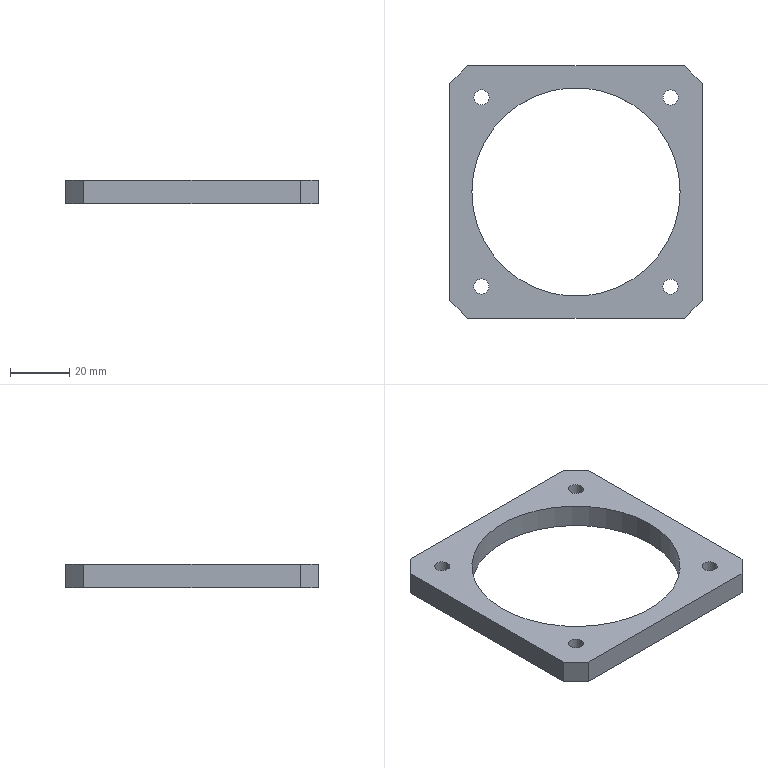Part | NX | 1 solid | 15 faces | box 85 x 85 x 8 mm | volume 25695 mm3 | plane 10 | cylinder 5 | commonest cylinder face diameters 5.1 x4 70.1 x1
STEP:
#1=CARTESIAN_POINT('',(-36.5,-42.5,0.));
#2=VERTEX_POINT('',#1);
#3=CARTESIAN_POINT('',(36.5,-42.5,0.));
#4=VERTEX_POINT('',#3);
#5=CARTESIAN_POINT('',(-36.5,-42.5,0.));
#6=DIRECTION('',(1.,0.,0.));
#7=VECTOR('',#6,1000.);
#8=LINE('',#5,#7);
#9=EDGE_CURVE('',#2,#4,#8,.T.);
#10=ORIENTED_EDGE('',*,*,#9,.F.);
#11=CARTESIAN_POINT('',(-36.5,-42.5,-8.));
#12=VERTEX_POINT('',#11);
#13=CARTESIAN_POINT('',(-36.5,-42.5,-8.));
#14=DIRECTION('',(0.,0.,1.));
#15=VECTOR('',#14,1000.);
#16=LINE('',#13,#15);
#17=EDGE_CURVE('',#12,#2,#16,.T.);
#18=ORIENTED_EDGE('',*,*,#17,.F.);
#19=CARTESIAN_POINT('',(36.5,-42.5,-8.));
#20=VERTEX_POINT('',#19);
#21=CARTESIAN_POINT('',(-36.5,-42.5,-8.));
#22=DIRECTION('',(1.,0.,0.));
#23=VECTOR('',#22,1000.);
#24=LINE('',#21,#23);
#25=EDGE_CURVE('',#12,#20,#24,.T.);
#26=ORIENTED_EDGE('',*,*,#25,.T.);
#27=CARTESIAN_POINT('',(36.5,-42.5,-8.));
#28=DIRECTION('',(0.,0.,1.));
#29=VECTOR('',#28,1000.);
#30=LINE('',#27,#29);
#31=EDGE_CURVE('',#20,#4,#30,.T.);
#32=ORIENTED_EDGE('',*,*,#31,.T.);
#33=EDGE_LOOP('',(#10,#18,#26,#32));
#34=FACE_BOUND('',#33,.T.);
#35=CARTESIAN_POINT('',(-36.5,-42.5,-8.));
#36=DIRECTION('',(0.,-1.,0.));
#37=DIRECTION('',(1.,0.,0.));
#38=AXIS2_PLACEMENT_3D('',#35,#36,#37);
#39=PLANE('',#38);
#40=ADVANCED_FACE('',(#34),#39,.T.);
#41=CARTESIAN_POINT('',(42.5,-36.5,0.));
#42=VERTEX_POINT('',#41);
#43=CARTESIAN_POINT('',(36.5,-42.5,0.));
#44=DIRECTION('',(0.7071,0.7071,0.));
#45=VECTOR('',#44,1000.);
#46=LINE('',#43,#45);
#47=EDGE_CURVE('',#4,#42,#46,.T.);
#48=ORIENTED_EDGE('',*,*,#47,.F.);
#49=ORIENTED_EDGE('',*,*,#31,.F.);
#50=CARTESIAN_POINT('',(42.5,-36.5,-8.));
#51=VERTEX_POINT('',#50);
#52=CARTESIAN_POINT('',(36.5,-42.5,-8.));
#53=DIRECTION('',(0.7071,0.7071,0.));
#54=VECTOR('',#53,1000.);
#55=LINE('',#52,#54);
#56=EDGE_CURVE('',#20,#51,#55,.T.);
#57=ORIENTED_EDGE('',*,*,#56,.T.);
#58=CARTESIAN_POINT('',(42.5,-36.5,-8.));
#59=DIRECTION('',(0.,0.,1.));
#60=VECTOR('',#59,1000.);
#61=LINE('',#58,#60);
#62=EDGE_CURVE('',#51,#42,#61,.T.);
#63=ORIENTED_EDGE('',*,*,#62,.T.);
#64=EDGE_LOOP('',(#48,#49,#57,#63));
#65=FACE_BOUND('',#64,.T.);
#66=CARTESIAN_POINT('',(36.5,-42.5,-8.));
#67=DIRECTION('',(0.7071,-0.7071,0.));
#68=DIRECTION('',(0.7071,0.7071,0.));
#69=AXIS2_PLACEMENT_3D('',#66,#67,#68);
#70=PLANE('',#69);
#71=ADVANCED_FACE('',(#65),#70,.T.);
#72=CARTESIAN_POINT('',(42.5,36.5,0.));
#73=VERTEX_POINT('',#72);
#74=CARTESIAN_POINT('',(42.5,-36.5,0.));
#75=DIRECTION('',(0.,1.,0.));
#76=VECTOR('',#75,1000.);
#77=LINE('',#74,#76);
#78=EDGE_CURVE('',#42,#73,#77,.T.);
#79=ORIENTED_EDGE('',*,*,#78,.F.);
#80=ORIENTED_EDGE('',*,*,#62,.F.);
#81=CARTESIAN_POINT('',(42.5,36.5,-8.));
#82=VERTEX_POINT('',#81);
#83=CARTESIAN_POINT('',(42.5,-36.5,-8.));
#84=DIRECTION('',(0.,1.,0.));
#85=VECTOR('',#84,1000.);
#86=LINE('',#83,#85);
#87=EDGE_CURVE('',#51,#82,#86,.T.);
#88=ORIENTED_EDGE('',*,*,#87,.T.);
#89=CARTESIAN_POINT('',(42.5,36.5,-8.));
#90=DIRECTION('',(0.,0.,1.));
#91=VECTOR('',#90,1000.);
#92=LINE('',#89,#91);
#93=EDGE_CURVE('',#82,#73,#92,.T.);
#94=ORIENTED_EDGE('',*,*,#93,.T.);
#95=EDGE_LOOP('',(#79,#80,#88,#94));
#96=FACE_BOUND('',#95,.T.);
#97=CARTESIAN_POINT('',(42.5,-36.5,-8.));
#98=DIRECTION('',(1.,0.,0.));
#99=DIRECTION('',(0.,1.,0.));
#100=AXIS2_PLACEMENT_3D('',#97,#98,#99);
#101=PLANE('',#100);
#102=ADVANCED_FACE('',(#96),#101,.T.);
#103=CARTESIAN_POINT('',(36.5,42.5,0.));
#104=VERTEX_POINT('',#103);
#105=CARTESIAN_POINT('',(42.5,36.5,0.));
#106=DIRECTION('',(-0.7071,0.7071,0.));
#107=VECTOR('',#106,1000.);
#108=LINE('',#105,#107);
#109=EDGE_CURVE('',#73,#104,#108,.T.);
#110=ORIENTED_EDGE('',*,*,#109,.F.);
#111=ORIENTED_EDGE('',*,*,#93,.F.);
#112=CARTESIAN_POINT('',(36.5,42.5,-8.));
#113=VERTEX_POINT('',#112);
#114=CARTESIAN_POINT('',(42.5,36.5,-8.));
#115=DIRECTION('',(-0.7071,0.7071,0.));
#116=VECTOR('',#115,1000.);
#117=LINE('',#114,#116);
#118=EDGE_CURVE('',#82,#113,#117,.T.);
#119=ORIENTED_EDGE('',*,*,#118,.T.);
#120=CARTESIAN_POINT('',(36.5,42.5,-8.));
#121=DIRECTION('',(0.,0.,1.));
#122=VECTOR('',#121,1000.);
#123=LINE('',#120,#122);
#124=EDGE_CURVE('',#113,#104,#123,.T.);
#125=ORIENTED_EDGE('',*,*,#124,.T.);
#126=EDGE_LOOP('',(#110,#111,#119,#125));
#127=FACE_BOUND('',#126,.T.);
#128=CARTESIAN_POINT('',(42.5,36.5,-8.));
#129=DIRECTION('',(0.7071,0.7071,0.));
#130=DIRECTION('',(-0.7071,0.7071,0.));
#131=AXIS2_PLACEMENT_3D('',#128,#129,#130);
#132=PLANE('',#131);
#133=ADVANCED_FACE('',(#127),#132,.T.);
#134=CARTESIAN_POINT('',(-36.5,42.5,0.));
#135=VERTEX_POINT('',#134);
#136=CARTESIAN_POINT('',(36.5,42.5,0.));
#137=DIRECTION('',(-1.,0.,0.));
#138=VECTOR('',#137,1000.);
#139=LINE('',#136,#138);
#140=EDGE_CURVE('',#104,#135,#139,.T.);
#141=ORIENTED_EDGE('',*,*,#140,.F.);
#142=ORIENTED_EDGE('',*,*,#124,.F.);
#143=CARTESIAN_POINT('',(-36.5,42.5,-8.));
#144=VERTEX_POINT('',#143);
#145=CARTESIAN_POINT('',(36.5,42.5,-8.));
#146=DIRECTION('',(-1.,0.,0.));
#147=VECTOR('',#146,1000.);
#148=LINE('',#145,#147);
#149=EDGE_CURVE('',#113,#144,#148,.T.);
#150=ORIENTED_EDGE('',*,*,#149,.T.);
#151=CARTESIAN_POINT('',(-36.5,42.5,-8.));
#152=DIRECTION('',(0.,0.,1.));
#153=VECTOR('',#152,1000.);
#154=LINE('',#151,#153);
#155=EDGE_CURVE('',#144,#135,#154,.T.);
#156=ORIENTED_EDGE('',*,*,#155,.T.);
#157=EDGE_LOOP('',(#141,#142,#150,#156));
#158=FACE_BOUND('',#157,.T.);
#159=CARTESIAN_POINT('',(36.5,42.5,-8.));
#160=DIRECTION('',(0.,1.,0.));
#161=DIRECTION('',(-1.,0.,0.));
#162=AXIS2_PLACEMENT_3D('',#159,#160,#161);
#163=PLANE('',#162);
#164=ADVANCED_FACE('',(#158),#163,.T.);
#165=CARTESIAN_POINT('',(-42.5,36.5,0.));
#166=VERTEX_POINT('',#165);
#167=CARTESIAN_POINT('',(-36.5,42.5,0.));
#168=DIRECTION('',(-0.7071,-0.7071,0.));
#169=VECTOR('',#168,1000.);
#170=LINE('',#167,#169);
#171=EDGE_CURVE('',#135,#166,#170,.T.);
#172=ORIENTED_EDGE('',*,*,#171,.F.);
#173=ORIENTED_EDGE('',*,*,#155,.F.);
#174=CARTESIAN_POINT('',(-42.5,36.5,-8.));
#175=VERTEX_POINT('',#174);
#176=CARTESIAN_POINT('',(-36.5,42.5,-8.));
#177=DIRECTION('',(-0.7071,-0.7071,0.));
#178=VECTOR('',#177,1000.);
#179=LINE('',#176,#178);
#180=EDGE_CURVE('',#144,#175,#179,.T.);
#181=ORIENTED_EDGE('',*,*,#180,.T.);
#182=CARTESIAN_POINT('',(-42.5,36.5,-8.));
#183=DIRECTION('',(0.,0.,1.));
#184=VECTOR('',#183,1000.);
#185=LINE('',#182,#184);
#186=EDGE_CURVE('',#175,#166,#185,.T.);
#187=ORIENTED_EDGE('',*,*,#186,.T.);
#188=EDGE_LOOP('',(#172,#173,#181,#187));
#189=FACE_BOUND('',#188,.T.);
#190=CARTESIAN_POINT('',(-36.5,42.5,-8.));
#191=DIRECTION('',(-0.7071,0.7071,0.));
#192=DIRECTION('',(-0.7071,-0.7071,0.));
#193=AXIS2_PLACEMENT_3D('',#190,#191,#192);
#194=PLANE('',#193);
#195=ADVANCED_FACE('',(#189),#194,.T.);
#196=CARTESIAN_POINT('',(-42.5,-36.5,0.));
#197=VERTEX_POINT('',#196);
#198=CARTESIAN_POINT('',(-42.5,36.5,0.));
#199=DIRECTION('',(0.,-1.,0.));
#200=VECTOR('',#199,1000.);
#201=LINE('',#198,#200);
#202=EDGE_CURVE('',#166,#197,#201,.T.);
#203=ORIENTED_EDGE('',*,*,#202,.F.);
#204=ORIENTED_EDGE('',*,*,#186,.F.);
#205=CARTESIAN_POINT('',(-42.5,-36.5,-8.));
#206=VERTEX_POINT('',#205);
#207=CARTESIAN_POINT('',(-42.5,36.5,-8.));
#208=DIRECTION('',(0.,-1.,0.));
#209=VECTOR('',#208,1000.);
#210=LINE('',#207,#209);
#211=EDGE_CURVE('',#175,#206,#210,.T.);
#212=ORIENTED_EDGE('',*,*,#211,.T.);
#213=CARTESIAN_POINT('',(-42.5,-36.5,-8.));
#214=DIRECTION('',(0.,0.,1.));
#215=VECTOR('',#214,1000.);
#216=LINE('',#213,#215);
#217=EDGE_CURVE('',#206,#197,#216,.T.);
#218=ORIENTED_EDGE('',*,*,#217,.T.);
#219=EDGE_LOOP('',(#203,#204,#212,#218));
#220=FACE_BOUND('',#219,.T.);
#221=CARTESIAN_POINT('',(-42.5,36.5,-8.));
#222=DIRECTION('',(-1.,0.,0.));
#223=DIRECTION('',(0.,-1.,0.));
#224=AXIS2_PLACEMENT_3D('',#221,#222,#223);
#225=PLANE('',#224);
#226=ADVANCED_FACE('',(#220),#225,.T.);
#227=CARTESIAN_POINT('',(29.27,-31.82,-8.));
#228=VERTEX_POINT('',#227);
#229=CARTESIAN_POINT('',(31.82,-31.82,-8.));
#230=DIRECTION('',(0.,0.,1.));
#231=DIRECTION('',(-1.,0.,0.));
#232=AXIS2_PLACEMENT_3D('',#229,#230,#231);
#233=CIRCLE('',#232,2.55);
#234=EDGE_CURVE('',#228,#228,#233,.T.);
#235=ORIENTED_EDGE('',*,*,#234,.F.);
#236=EDGE_LOOP('',(#235));
#237=FACE_BOUND('',#236,.T.);
#238=CARTESIAN_POINT('',(29.27,-31.82,0.));
#239=VERTEX_POINT('',#238);
#240=CARTESIAN_POINT('',(31.82,-31.82,0.));
#241=DIRECTION('',(0.,0.,1.));
#242=DIRECTION('',(-1.,0.,0.));
#243=AXIS2_PLACEMENT_3D('',#240,#241,#242);
#244=CIRCLE('',#243,2.55);
#245=EDGE_CURVE('',#239,#239,#244,.T.);
#246=ORIENTED_EDGE('',*,*,#245,.T.);
#247=EDGE_LOOP('',(#246));
#248=FACE_BOUND('',#247,.T.);
#249=CARTESIAN_POINT('',(31.82,-31.82,-8.));
#250=DIRECTION('',(0.,0.,1.));
#251=DIRECTION('',(1.,0.,0.));
#252=AXIS2_PLACEMENT_3D('',#249,#250,#251);
#253=CYLINDRICAL_SURFACE('',#252,2.55);
#254=ADVANCED_FACE('',(#237,#248),#253,.F.);
#255=CARTESIAN_POINT('',(-29.27,31.82,-8.));
#256=VERTEX_POINT('',#255);
#257=CARTESIAN_POINT('',(-31.82,31.82,-8.));
#258=DIRECTION('',(0.,0.,1.));
#259=DIRECTION('',(1.,0.,0.));
#260=AXIS2_PLACEMENT_3D('',#257,#258,#259);
#261=CIRCLE('',#260,2.55);
#262=EDGE_CURVE('',#256,#256,#261,.T.);
#263=ORIENTED_EDGE('',*,*,#262,.F.);
#264=EDGE_LOOP('',(#263));
#265=FACE_BOUND('',#264,.T.);
#266=CARTESIAN_POINT('',(-29.27,31.82,0.));
#267=VERTEX_POINT('',#266);
#268=CARTESIAN_POINT('',(-31.82,31.82,0.));
#269=DIRECTION('',(0.,0.,1.));
#270=DIRECTION('',(1.,0.,0.));
#271=AXIS2_PLACEMENT_3D('',#268,#269,#270);
#272=CIRCLE('',#271,2.55);
#273=EDGE_CURVE('',#267,#267,#272,.T.);
#274=ORIENTED_EDGE('',*,*,#273,.T.);
#275=EDGE_LOOP('',(#274));
#276=FACE_BOUND('',#275,.T.);
#277=CARTESIAN_POINT('',(-31.82,31.82,-8.));
#278=DIRECTION('',(0.,0.,1.));
#279=DIRECTION('',(1.,0.,0.));
#280=AXIS2_PLACEMENT_3D('',#277,#278,#279);
#281=CYLINDRICAL_SURFACE('',#280,2.55);
#282=ADVANCED_FACE('',(#265,#276),#281,.F.);
#283=CARTESIAN_POINT('',(-31.82,-29.27,-8.));
#284=VERTEX_POINT('',#283);
#285=CARTESIAN_POINT('',(-31.82,-31.82,-8.));
#286=DIRECTION('',(0.,0.,1.));
#287=DIRECTION('',(0.,1.,0.));
#288=AXIS2_PLACEMENT_3D('',#285,#286,#287);
#289=CIRCLE('',#288,2.55);
#290=EDGE_CURVE('',#284,#284,#289,.T.);
#291=ORIENTED_EDGE('',*,*,#290,.F.);
#292=EDGE_LOOP('',(#291));
#293=FACE_BOUND('',#292,.T.);
#294=CARTESIAN_POINT('',(-31.82,-29.27,0.));
#295=VERTEX_POINT('',#294);
#296=CARTESIAN_POINT('',(-31.82,-31.82,0.));
#297=DIRECTION('',(0.,0.,1.));
#298=DIRECTION('',(0.,1.,0.));
#299=AXIS2_PLACEMENT_3D('',#296,#297,#298);
#300=CIRCLE('',#299,2.55);
#301=EDGE_CURVE('',#295,#295,#300,.T.);
#302=ORIENTED_EDGE('',*,*,#301,.T.);
#303=EDGE_LOOP('',(#302));
#304=FACE_BOUND('',#303,.T.);
#305=CARTESIAN_POINT('',(-31.82,-31.82,-8.));
#306=DIRECTION('',(0.,0.,1.));
#307=DIRECTION('',(1.,0.,0.));
#308=AXIS2_PLACEMENT_3D('',#305,#306,#307);
#309=CYLINDRICAL_SURFACE('',#308,2.55);
#310=ADVANCED_FACE('',(#293,#304),#309,.F.);
#311=CARTESIAN_POINT('',(35.05,0.,-8.));
#312=VERTEX_POINT('',#311);
#313=CARTESIAN_POINT('',(0.,0.,-8.));
#314=DIRECTION('',(0.,0.,1.));
#315=DIRECTION('',(1.,0.,0.));
#316=AXIS2_PLACEMENT_3D('',#313,#314,#315);
#317=CIRCLE('',#316,35.05);
#318=EDGE_CURVE('',#312,#312,#317,.T.);
#319=ORIENTED_EDGE('',*,*,#318,.F.);
#320=EDGE_LOOP('',(#319));
#321=FACE_BOUND('',#320,.T.);
#322=CARTESIAN_POINT('',(35.05,0.,0.));
#323=VERTEX_POINT('',#322);
#324=CARTESIAN_POINT('',(0.,0.,0.));
#325=DIRECTION('',(0.,0.,1.));
#326=DIRECTION('',(1.,0.,0.));
#327=AXIS2_PLACEMENT_3D('',#324,#325,#326);
#328=CIRCLE('',#327,35.05);
#329=EDGE_CURVE('',#323,#323,#328,.T.);
#330=ORIENTED_EDGE('',*,*,#329,.T.);
#331=EDGE_LOOP('',(#330));
#332=FACE_BOUND('',#331,.T.);
#333=CARTESIAN_POINT('',(0.,0.,-8.));
#334=DIRECTION('',(0.,0.,1.));
#335=DIRECTION('',(1.,0.,0.));
#336=AXIS2_PLACEMENT_3D('',#333,#334,#335);
#337=CYLINDRICAL_SURFACE('',#336,35.05);
#338=ADVANCED_FACE('',(#321,#332),#337,.F.);
#339=CARTESIAN_POINT('',(-42.5,-36.5,0.));
#340=DIRECTION('',(0.7071,-0.7071,0.));
#341=VECTOR('',#340,1000.);
#342=LINE('',#339,#341);
#343=EDGE_CURVE('',#197,#2,#342,.T.);
#344=ORIENTED_EDGE('',*,*,#343,.F.);
#345=ORIENTED_EDGE('',*,*,#217,.F.);
#346=CARTESIAN_POINT('',(-42.5,-36.5,-8.));
#347=DIRECTION('',(0.7071,-0.7071,0.));
#348=VECTOR('',#347,1000.);
#349=LINE('',#346,#348);
#350=EDGE_CURVE('',#206,#12,#349,.T.);
#351=ORIENTED_EDGE('',*,*,#350,.T.);
#352=ORIENTED_EDGE('',*,*,#17,.T.);
#353=EDGE_LOOP('',(#344,#345,#351,#352));
#354=FACE_BOUND('',#353,.T.);
#355=CARTESIAN_POINT('',(-42.5,-36.5,-8.));
#356=DIRECTION('',(-0.7071,-0.7071,0.));
#357=DIRECTION('',(0.7071,-0.7071,0.));
#358=AXIS2_PLACEMENT_3D('',#355,#356,#357);
#359=PLANE('',#358);
#360=ADVANCED_FACE('',(#354),#359,.T.);
#361=CARTESIAN_POINT('',(31.82,29.27,-8.));
#362=VERTEX_POINT('',#361);
#363=CARTESIAN_POINT('',(31.82,31.82,-8.));
#364=DIRECTION('',(0.,0.,1.));
#365=DIRECTION('',(0.,-1.,0.));
#366=AXIS2_PLACEMENT_3D('',#363,#364,#365);
#367=CIRCLE('',#366,2.55);
#368=EDGE_CURVE('',#362,#362,#367,.T.);
#369=ORIENTED_EDGE('',*,*,#368,.F.);
#370=EDGE_LOOP('',(#369));
#371=FACE_BOUND('',#370,.T.);
#372=CARTESIAN_POINT('',(31.82,29.27,0.));
#373=VERTEX_POINT('',#372);
#374=CARTESIAN_POINT('',(31.82,31.82,0.));
#375=DIRECTION('',(0.,0.,1.));
#376=DIRECTION('',(0.,-1.,0.));
#377=AXIS2_PLACEMENT_3D('',#374,#375,#376);
#378=CIRCLE('',#377,2.55);
#379=EDGE_CURVE('',#373,#373,#378,.T.);
#380=ORIENTED_EDGE('',*,*,#379,.T.);
#381=EDGE_LOOP('',(#380));
#382=FACE_BOUND('',#381,.T.);
#383=CARTESIAN_POINT('',(31.82,31.82,-8.));
#384=DIRECTION('',(0.,0.,1.));
#385=DIRECTION('',(1.,0.,0.));
#386=AXIS2_PLACEMENT_3D('',#383,#384,#385);
#387=CYLINDRICAL_SURFACE('',#386,2.55);
#388=ADVANCED_FACE('',(#371,#382),#387,.F.);
#389=ORIENTED_EDGE('',*,*,#25,.F.);
#390=ORIENTED_EDGE('',*,*,#350,.F.);
#391=ORIENTED_EDGE('',*,*,#211,.F.);
#392=ORIENTED_EDGE('',*,*,#180,.F.);
#393=ORIENTED_EDGE('',*,*,#149,.F.);
#394=ORIENTED_EDGE('',*,*,#118,.F.);
#395=ORIENTED_EDGE('',*,*,#87,.F.);
#396=ORIENTED_EDGE('',*,*,#56,.F.);
#397=EDGE_LOOP('',(#389,#390,#391,#392,#393,#394,#395,#396));
#398=FACE_BOUND('',#397,.T.);
#399=ORIENTED_EDGE('',*,*,#318,.T.);
#400=EDGE_LOOP('',(#399));
#401=FACE_BOUND('',#400,.T.);
#402=ORIENTED_EDGE('',*,*,#290,.T.);
#403=EDGE_LOOP('',(#402));
#404=FACE_BOUND('',#403,.T.);
#405=ORIENTED_EDGE('',*,*,#262,.T.);
#406=EDGE_LOOP('',(#405));
#407=FACE_BOUND('',#406,.T.);
#408=ORIENTED_EDGE('',*,*,#234,.T.);
#409=EDGE_LOOP('',(#408));
#410=FACE_BOUND('',#409,.T.);
#411=ORIENTED_EDGE('',*,*,#368,.T.);
#412=EDGE_LOOP('',(#411));
#413=FACE_BOUND('',#412,.T.);
#414=CARTESIAN_POINT('',(0.,0.,-8.));
#415=DIRECTION('',(0.,0.,1.));
#416=DIRECTION('',(1.,0.,0.));
#417=AXIS2_PLACEMENT_3D('',#414,#415,#416);
#418=PLANE('',#417);
#419=ADVANCED_FACE('',(#398,#401,#404,#407,#410,#413),#418,.F.);
#420=ORIENTED_EDGE('',*,*,#9,.T.);
#421=ORIENTED_EDGE('',*,*,#47,.T.);
#422=ORIENTED_EDGE('',*,*,#78,.T.);
#423=ORIENTED_EDGE('',*,*,#109,.T.);
#424=ORIENTED_EDGE('',*,*,#140,.T.);
#425=ORIENTED_EDGE('',*,*,#171,.T.);
#426=ORIENTED_EDGE('',*,*,#202,.T.);
#427=ORIENTED_EDGE('',*,*,#343,.T.);
#428=EDGE_LOOP('',(#420,#421,#422,#423,#424,#425,#426,#427));
#429=FACE_BOUND('',#428,.T.);
#430=ORIENTED_EDGE('',*,*,#329,.F.);
#431=EDGE_LOOP('',(#430));
#432=FACE_BOUND('',#431,.T.);
#433=ORIENTED_EDGE('',*,*,#301,.F.);
#434=EDGE_LOOP('',(#433));
#435=FACE_BOUND('',#434,.T.);
#436=ORIENTED_EDGE('',*,*,#273,.F.);
#437=EDGE_LOOP('',(#436));
#438=FACE_BOUND('',#437,.T.);
#439=ORIENTED_EDGE('',*,*,#245,.F.);
#440=EDGE_LOOP('',(#439));
#441=FACE_BOUND('',#440,.T.);
#442=ORIENTED_EDGE('',*,*,#379,.F.);
#443=EDGE_LOOP('',(#442));
#444=FACE_BOUND('',#443,.T.);
#445=CARTESIAN_POINT('',(0.,0.,0.));
#446=DIRECTION('',(0.,0.,1.));
#447=DIRECTION('',(1.,0.,0.));
#448=AXIS2_PLACEMENT_3D('',#445,#446,#447);
#449=PLANE('',#448);
#450=ADVANCED_FACE('',(#429,#432,#435,#438,#441,#444),#449,.T.);
#451=CLOSED_SHELL('',(#40,#71,#102,#133,#164,#195,#226,#254,#282,#310,#338,#360,#388,#419,#450));
#452=MANIFOLD_SOLID_BREP('',#451);
#453=(LENGTH_UNIT()NAMED_UNIT(*)SI_UNIT(.MILLI.,.METRE.));
#454=UNCERTAINTY_MEASURE_WITH_UNIT(LENGTH_MEASURE(0.00001),#453,'','');
#455=(NAMED_UNIT(*)PLANE_ANGLE_UNIT()SI_UNIT($,.RADIAN.));
#456=(NAMED_UNIT(*)SI_UNIT($,.STERADIAN.)SOLID_ANGLE_UNIT());
#457=(GEOMETRIC_REPRESENTATION_CONTEXT(3)GLOBAL_UNCERTAINTY_ASSIGNED_CONTEXT((#454))GLOBAL_UNIT_ASSIGNED_CONTEXT((#453,#455,#456))REPRESENTATION_CONTEXT('',''));
#458=ADVANCED_BREP_SHAPE_REPRESENTATION('',(#452),#457);